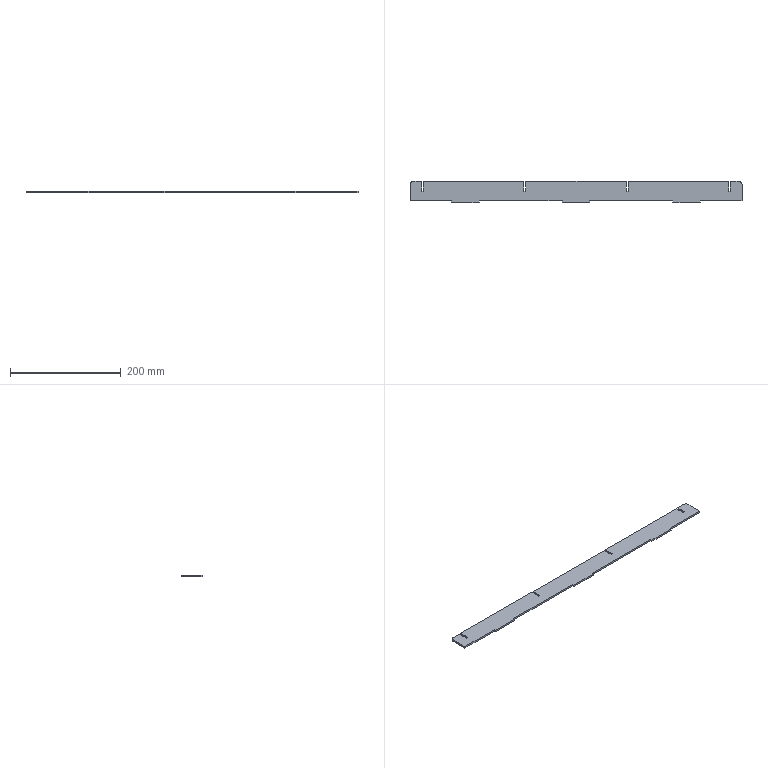Part | SolidWorks | features FlatPattern 1, SMBaseFlange 1, SheetMetal 1 | 1 solid | 36 faces | box 600 x 38 x 3.2 mm | volume 67879 mm3 | plane 34 | cylinder 2 | commonest cylinder face diameters 10 x2
STEP:
#1=CARTESIAN_POINT('',(254.609,-214.8,0.));
#2=VERTEX_POINT('',#1);
#3=CARTESIAN_POINT('',(254.609,-184.8,0.));
#4=VERTEX_POINT('',#3);
#5=CARTESIAN_POINT('',(254.609,-214.8,0.));
#6=DIRECTION('',(0.,1.,0.));
#7=VECTOR('',#6,1000.);
#8=LINE('',#5,#7);
#9=EDGE_CURVE('',#2,#4,#8,.T.);
#10=ORIENTED_EDGE('',*,*,#9,.F.);
#11=CARTESIAN_POINT('',(254.609,-214.8,-3.2));
#12=VERTEX_POINT('',#11);
#13=CARTESIAN_POINT('',(254.609,-214.8,-3.2));
#14=DIRECTION('',(0.,0.,1.));
#15=VECTOR('',#14,1000.);
#16=LINE('',#13,#15);
#17=EDGE_CURVE('',#12,#2,#16,.T.);
#18=ORIENTED_EDGE('',*,*,#17,.F.);
#19=CARTESIAN_POINT('',(254.609,-184.8,-3.2));
#20=VERTEX_POINT('',#19);
#21=CARTESIAN_POINT('',(254.609,-214.8,-3.2));
#22=DIRECTION('',(0.,1.,0.));
#23=VECTOR('',#22,1000.);
#24=LINE('',#21,#23);
#25=EDGE_CURVE('',#12,#20,#24,.T.);
#26=ORIENTED_EDGE('',*,*,#25,.T.);
#27=CARTESIAN_POINT('',(254.609,-184.8,-3.2));
#28=DIRECTION('',(0.,0.,1.));
#29=VECTOR('',#28,1000.);
#30=LINE('',#27,#29);
#31=EDGE_CURVE('',#20,#4,#30,.T.);
#32=ORIENTED_EDGE('',*,*,#31,.T.);
#33=EDGE_LOOP('',(#10,#18,#26,#32));
#34=FACE_OUTER_BOUND('',#33,.T.);
#35=CARTESIAN_POINT('',(254.609,-214.8,-3.2));
#36=DIRECTION('',(1.,0.,0.));
#37=DIRECTION('',(0.,0.,-1.));
#38=AXIS2_PLACEMENT_3D('',#35,#36,#37);
#39=PLANE('',#38);
#40=ADVANCED_FACE('',(#34),#39,.T.);
#41=CARTESIAN_POINT('',(179.609,-214.8,0.));
#42=VERTEX_POINT('',#41);
#43=CARTESIAN_POINT('',(254.609,-214.8,0.));
#44=DIRECTION('',(1.,0.,0.));
#45=VECTOR('',#44,1000.);
#46=LINE('',#43,#45);
#47=EDGE_CURVE('',#42,#2,#46,.T.);
#48=ORIENTED_EDGE('',*,*,#47,.F.);
#49=CARTESIAN_POINT('',(179.609,-214.8,-3.2));
#50=VERTEX_POINT('',#49);
#51=CARTESIAN_POINT('',(179.609,-214.8,-3.2));
#52=DIRECTION('',(0.,0.,1.));
#53=VECTOR('',#52,1000.);
#54=LINE('',#51,#53);
#55=EDGE_CURVE('',#50,#42,#54,.T.);
#56=ORIENTED_EDGE('',*,*,#55,.F.);
#57=CARTESIAN_POINT('',(254.609,-214.8,-3.2));
#58=DIRECTION('',(1.,0.,0.));
#59=VECTOR('',#58,1000.);
#60=LINE('',#57,#59);
#61=EDGE_CURVE('',#50,#12,#60,.T.);
#62=ORIENTED_EDGE('',*,*,#61,.T.);
#63=ORIENTED_EDGE('',*,*,#17,.T.);
#64=EDGE_LOOP('',(#48,#56,#62,#63));
#65=FACE_OUTER_BOUND('',#64,.T.);
#66=CARTESIAN_POINT('',(254.609,-214.8,-3.2));
#67=DIRECTION('',(0.,-1.,0.));
#68=DIRECTION('',(1.,0.,0.));
#69=AXIS2_PLACEMENT_3D('',#66,#67,#68);
#70=PLANE('',#69);
#71=ADVANCED_FACE('',(#65),#70,.T.);
#72=CARTESIAN_POINT('',(179.609,-217.8,0.));
#73=VERTEX_POINT('',#72);
#74=CARTESIAN_POINT('',(179.609,-214.8,0.));
#75=DIRECTION('',(0.,1.,0.));
#76=VECTOR('',#75,1000.);
#77=LINE('',#74,#76);
#78=EDGE_CURVE('',#73,#42,#77,.T.);
#79=ORIENTED_EDGE('',*,*,#78,.F.);
#80=CARTESIAN_POINT('',(179.609,-217.8,-3.2));
#81=VERTEX_POINT('',#80);
#82=CARTESIAN_POINT('',(179.609,-217.8,-3.2));
#83=DIRECTION('',(0.,0.,1.));
#84=VECTOR('',#83,1000.);
#85=LINE('',#82,#84);
#86=EDGE_CURVE('',#81,#73,#85,.T.);
#87=ORIENTED_EDGE('',*,*,#86,.F.);
#88=CARTESIAN_POINT('',(179.609,-214.8,-3.2));
#89=DIRECTION('',(0.,1.,0.));
#90=VECTOR('',#89,1000.);
#91=LINE('',#88,#90);
#92=EDGE_CURVE('',#81,#50,#91,.T.);
#93=ORIENTED_EDGE('',*,*,#92,.T.);
#94=ORIENTED_EDGE('',*,*,#55,.T.);
#95=EDGE_LOOP('',(#79,#87,#93,#94));
#96=FACE_OUTER_BOUND('',#95,.T.);
#97=CARTESIAN_POINT('',(179.609,-214.8,-3.2));
#98=DIRECTION('',(1.,0.,0.));
#99=DIRECTION('',(0.,0.,-1.));
#100=AXIS2_PLACEMENT_3D('',#97,#98,#99);
#101=PLANE('',#100);
#102=ADVANCED_FACE('',(#96),#101,.T.);
#103=CARTESIAN_POINT('',(129.609,-217.8,0.));
#104=VERTEX_POINT('',#103);
#105=CARTESIAN_POINT('',(179.609,-217.8,0.));
#106=DIRECTION('',(1.,0.,0.));
#107=VECTOR('',#106,1000.);
#108=LINE('',#105,#107);
#109=EDGE_CURVE('',#104,#73,#108,.T.);
#110=ORIENTED_EDGE('',*,*,#109,.F.);
#111=CARTESIAN_POINT('',(129.609,-217.8,-3.2));
#112=VERTEX_POINT('',#111);
#113=CARTESIAN_POINT('',(129.609,-217.8,-3.2));
#114=DIRECTION('',(0.,0.,1.));
#115=VECTOR('',#114,1000.);
#116=LINE('',#113,#115);
#117=EDGE_CURVE('',#112,#104,#116,.T.);
#118=ORIENTED_EDGE('',*,*,#117,.F.);
#119=CARTESIAN_POINT('',(179.609,-217.8,-3.2));
#120=DIRECTION('',(1.,0.,0.));
#121=VECTOR('',#120,1000.);
#122=LINE('',#119,#121);
#123=EDGE_CURVE('',#112,#81,#122,.T.);
#124=ORIENTED_EDGE('',*,*,#123,.T.);
#125=ORIENTED_EDGE('',*,*,#86,.T.);
#126=EDGE_LOOP('',(#110,#118,#124,#125));
#127=FACE_OUTER_BOUND('',#126,.T.);
#128=CARTESIAN_POINT('',(179.609,-217.8,-3.2));
#129=DIRECTION('',(0.,-1.,0.));
#130=DIRECTION('',(1.,0.,0.));
#131=AXIS2_PLACEMENT_3D('',#128,#129,#130);
#132=PLANE('',#131);
#133=ADVANCED_FACE('',(#127),#132,.T.);
#134=CARTESIAN_POINT('',(129.609,-214.8,0.));
#135=VERTEX_POINT('',#134);
#136=CARTESIAN_POINT('',(129.609,-217.8,0.));
#137=DIRECTION('',(0.,-1.,0.));
#138=VECTOR('',#137,1000.);
#139=LINE('',#136,#138);
#140=EDGE_CURVE('',#135,#104,#139,.T.);
#141=ORIENTED_EDGE('',*,*,#140,.F.);
#142=CARTESIAN_POINT('',(129.609,-214.8,-3.2));
#143=VERTEX_POINT('',#142);
#144=CARTESIAN_POINT('',(129.609,-214.8,-3.2));
#145=DIRECTION('',(0.,0.,1.));
#146=VECTOR('',#145,1000.);
#147=LINE('',#144,#146);
#148=EDGE_CURVE('',#143,#135,#147,.T.);
#149=ORIENTED_EDGE('',*,*,#148,.F.);
#150=CARTESIAN_POINT('',(129.609,-217.8,-3.2));
#151=DIRECTION('',(0.,-1.,0.));
#152=VECTOR('',#151,1000.);
#153=LINE('',#150,#152);
#154=EDGE_CURVE('',#143,#112,#153,.T.);
#155=ORIENTED_EDGE('',*,*,#154,.T.);
#156=ORIENTED_EDGE('',*,*,#117,.T.);
#157=EDGE_LOOP('',(#141,#149,#155,#156));
#158=FACE_OUTER_BOUND('',#157,.T.);
#159=CARTESIAN_POINT('',(129.609,-217.8,-3.2));
#160=DIRECTION('',(-1.,0.,0.));
#161=DIRECTION('',(0.,0.,1.));
#162=AXIS2_PLACEMENT_3D('',#159,#160,#161);
#163=PLANE('',#162);
#164=ADVANCED_FACE('',(#158),#163,.T.);
#165=CARTESIAN_POINT('',(-20.391,-214.8,0.));
#166=VERTEX_POINT('',#165);
#167=CARTESIAN_POINT('',(129.609,-214.8,0.));
#168=DIRECTION('',(1.,0.,0.));
#169=VECTOR('',#168,1000.);
#170=LINE('',#167,#169);
#171=EDGE_CURVE('',#166,#135,#170,.T.);
#172=ORIENTED_EDGE('',*,*,#171,.F.);
#173=CARTESIAN_POINT('',(-20.391,-214.8,-3.2));
#174=VERTEX_POINT('',#173);
#175=CARTESIAN_POINT('',(-20.391,-214.8,-3.2));
#176=DIRECTION('',(0.,0.,1.));
#177=VECTOR('',#176,1000.);
#178=LINE('',#175,#177);
#179=EDGE_CURVE('',#174,#166,#178,.T.);
#180=ORIENTED_EDGE('',*,*,#179,.F.);
#181=CARTESIAN_POINT('',(129.609,-214.8,-3.2));
#182=DIRECTION('',(1.,0.,0.));
#183=VECTOR('',#182,1000.);
#184=LINE('',#181,#183);
#185=EDGE_CURVE('',#174,#143,#184,.T.);
#186=ORIENTED_EDGE('',*,*,#185,.T.);
#187=ORIENTED_EDGE('',*,*,#148,.T.);
#188=EDGE_LOOP('',(#172,#180,#186,#187));
#189=FACE_OUTER_BOUND('',#188,.T.);
#190=CARTESIAN_POINT('',(129.609,-214.8,-3.2));
#191=DIRECTION('',(0.,-1.,0.));
#192=DIRECTION('',(0.,0.,-1.));
#193=AXIS2_PLACEMENT_3D('',#190,#191,#192);
#194=PLANE('',#193);
#195=ADVANCED_FACE('',(#189),#194,.T.);
#196=CARTESIAN_POINT('',(-20.391,-217.8,0.));
#197=VERTEX_POINT('',#196);
#198=CARTESIAN_POINT('',(-20.391,-214.8,0.));
#199=DIRECTION('',(0.,1.,0.));
#200=VECTOR('',#199,1000.);
#201=LINE('',#198,#200);
#202=EDGE_CURVE('',#197,#166,#201,.T.);
#203=ORIENTED_EDGE('',*,*,#202,.F.);
#204=CARTESIAN_POINT('',(-20.391,-217.8,-3.2));
#205=VERTEX_POINT('',#204);
#206=CARTESIAN_POINT('',(-20.391,-217.8,-3.2));
#207=DIRECTION('',(0.,0.,1.));
#208=VECTOR('',#207,1000.);
#209=LINE('',#206,#208);
#210=EDGE_CURVE('',#205,#197,#209,.T.);
#211=ORIENTED_EDGE('',*,*,#210,.F.);
#212=CARTESIAN_POINT('',(-20.391,-214.8,-3.2));
#213=DIRECTION('',(0.,1.,0.));
#214=VECTOR('',#213,1000.);
#215=LINE('',#212,#214);
#216=EDGE_CURVE('',#205,#174,#215,.T.);
#217=ORIENTED_EDGE('',*,*,#216,.T.);
#218=ORIENTED_EDGE('',*,*,#179,.T.);
#219=EDGE_LOOP('',(#203,#211,#217,#218));
#220=FACE_OUTER_BOUND('',#219,.T.);
#221=CARTESIAN_POINT('',(-20.391,-214.8,-3.2));
#222=DIRECTION('',(1.,0.,0.));
#223=DIRECTION('',(0.,1.,0.));
#224=AXIS2_PLACEMENT_3D('',#221,#222,#223);
#225=PLANE('',#224);
#226=ADVANCED_FACE('',(#220),#225,.T.);
#227=CARTESIAN_POINT('',(-70.391,-217.8,0.));
#228=VERTEX_POINT('',#227);
#229=CARTESIAN_POINT('',(-20.391,-217.8,0.));
#230=DIRECTION('',(1.,0.,0.));
#231=VECTOR('',#230,1000.);
#232=LINE('',#229,#231);
#233=EDGE_CURVE('',#228,#197,#232,.T.);
#234=ORIENTED_EDGE('',*,*,#233,.F.);
#235=CARTESIAN_POINT('',(-70.391,-217.8,-3.2));
#236=VERTEX_POINT('',#235);
#237=CARTESIAN_POINT('',(-70.391,-217.8,-3.2));
#238=DIRECTION('',(0.,0.,1.));
#239=VECTOR('',#238,1000.);
#240=LINE('',#237,#239);
#241=EDGE_CURVE('',#236,#228,#240,.T.);
#242=ORIENTED_EDGE('',*,*,#241,.F.);
#243=CARTESIAN_POINT('',(-20.391,-217.8,-3.2));
#244=DIRECTION('',(1.,0.,0.));
#245=VECTOR('',#244,1000.);
#246=LINE('',#243,#245);
#247=EDGE_CURVE('',#236,#205,#246,.T.);
#248=ORIENTED_EDGE('',*,*,#247,.T.);
#249=ORIENTED_EDGE('',*,*,#210,.T.);
#250=EDGE_LOOP('',(#234,#242,#248,#249));
#251=FACE_OUTER_BOUND('',#250,.T.);
#252=CARTESIAN_POINT('',(-20.391,-217.8,-3.2));
#253=DIRECTION('',(0.,-1.,0.));
#254=DIRECTION('',(0.,0.,-1.));
#255=AXIS2_PLACEMENT_3D('',#252,#253,#254);
#256=PLANE('',#255);
#257=ADVANCED_FACE('',(#251),#256,.T.);
#258=CARTESIAN_POINT('',(-70.391,-214.8,0.));
#259=VERTEX_POINT('',#258);
#260=CARTESIAN_POINT('',(-70.391,-217.8,0.));
#261=DIRECTION('',(0.,-1.,0.));
#262=VECTOR('',#261,1000.);
#263=LINE('',#260,#262);
#264=EDGE_CURVE('',#259,#228,#263,.T.);
#265=ORIENTED_EDGE('',*,*,#264,.F.);
#266=CARTESIAN_POINT('',(-70.391,-214.8,-3.2));
#267=VERTEX_POINT('',#266);
#268=CARTESIAN_POINT('',(-70.391,-214.8,-3.2));
#269=DIRECTION('',(0.,0.,1.));
#270=VECTOR('',#269,1000.);
#271=LINE('',#268,#270);
#272=EDGE_CURVE('',#267,#259,#271,.T.);
#273=ORIENTED_EDGE('',*,*,#272,.F.);
#274=CARTESIAN_POINT('',(-70.391,-217.8,-3.2));
#275=DIRECTION('',(0.,-1.,0.));
#276=VECTOR('',#275,1000.);
#277=LINE('',#274,#276);
#278=EDGE_CURVE('',#267,#236,#277,.T.);
#279=ORIENTED_EDGE('',*,*,#278,.T.);
#280=ORIENTED_EDGE('',*,*,#241,.T.);
#281=EDGE_LOOP('',(#265,#273,#279,#280));
#282=FACE_OUTER_BOUND('',#281,.T.);
#283=CARTESIAN_POINT('',(-70.391,-217.8,-3.2));
#284=DIRECTION('',(-1.,0.,0.));
#285=DIRECTION('',(0.,0.,1.));
#286=AXIS2_PLACEMENT_3D('',#283,#284,#285);
#287=PLANE('',#286);
#288=ADVANCED_FACE('',(#282),#287,.T.);
#289=CARTESIAN_POINT('',(-220.391,-214.8,0.));
#290=VERTEX_POINT('',#289);
#291=CARTESIAN_POINT('',(-70.391,-214.8,0.));
#292=DIRECTION('',(1.,0.,0.));
#293=VECTOR('',#292,1000.);
#294=LINE('',#291,#293);
#295=EDGE_CURVE('',#290,#259,#294,.T.);
#296=ORIENTED_EDGE('',*,*,#295,.F.);
#297=CARTESIAN_POINT('',(-220.391,-214.8,-3.2));
#298=VERTEX_POINT('',#297);
#299=CARTESIAN_POINT('',(-220.391,-214.8,-3.2));
#300=DIRECTION('',(0.,0.,1.));
#301=VECTOR('',#300,1000.);
#302=LINE('',#299,#301);
#303=EDGE_CURVE('',#298,#290,#302,.T.);
#304=ORIENTED_EDGE('',*,*,#303,.F.);
#305=CARTESIAN_POINT('',(-70.391,-214.8,-3.2));
#306=DIRECTION('',(1.,0.,0.));
#307=VECTOR('',#306,1000.);
#308=LINE('',#305,#307);
#309=EDGE_CURVE('',#298,#267,#308,.T.);
#310=ORIENTED_EDGE('',*,*,#309,.T.);
#311=ORIENTED_EDGE('',*,*,#272,.T.);
#312=EDGE_LOOP('',(#296,#304,#310,#311));
#313=FACE_OUTER_BOUND('',#312,.T.);
#314=CARTESIAN_POINT('',(-70.391,-214.8,-3.2));
#315=DIRECTION('',(0.,-1.,0.));
#316=DIRECTION('',(0.,0.,-1.));
#317=AXIS2_PLACEMENT_3D('',#314,#315,#316);
#318=PLANE('',#317);
#319=ADVANCED_FACE('',(#313),#318,.T.);
#320=CARTESIAN_POINT('',(-220.391,-217.8,0.));
#321=VERTEX_POINT('',#320);
#322=CARTESIAN_POINT('',(-220.391,-217.8,0.));
#323=DIRECTION('',(0.,1.,0.));
#324=VECTOR('',#323,1000.);
#325=LINE('',#322,#324);
#326=EDGE_CURVE('',#321,#290,#325,.T.);
#327=ORIENTED_EDGE('',*,*,#326,.F.);
#328=CARTESIAN_POINT('',(-220.391,-217.8,-3.2));
#329=VERTEX_POINT('',#328);
#330=CARTESIAN_POINT('',(-220.391,-217.8,-3.2));
#331=DIRECTION('',(0.,0.,1.));
#332=VECTOR('',#331,1000.);
#333=LINE('',#330,#332);
#334=EDGE_CURVE('',#329,#321,#333,.T.);
#335=ORIENTED_EDGE('',*,*,#334,.F.);
#336=CARTESIAN_POINT('',(-220.391,-217.8,-3.2));
#337=DIRECTION('',(0.,1.,0.));
#338=VECTOR('',#337,1000.);
#339=LINE('',#336,#338);
#340=EDGE_CURVE('',#329,#298,#339,.T.);
#341=ORIENTED_EDGE('',*,*,#340,.T.);
#342=ORIENTED_EDGE('',*,*,#303,.T.);
#343=EDGE_LOOP('',(#327,#335,#341,#342));
#344=FACE_OUTER_BOUND('',#343,.T.);
#345=CARTESIAN_POINT('',(-220.391,-217.8,-3.2));
#346=DIRECTION('',(1.,0.,0.));
#347=DIRECTION('',(0.,1.,0.));
#348=AXIS2_PLACEMENT_3D('',#345,#346,#347);
#349=PLANE('',#348);
#350=ADVANCED_FACE('',(#344),#349,.T.);
#351=CARTESIAN_POINT('',(-270.391,-217.8,0.));
#352=VERTEX_POINT('',#351);
#353=CARTESIAN_POINT('',(-270.391,-217.8,0.));
#354=DIRECTION('',(1.,0.,0.));
#355=VECTOR('',#354,1000.);
#356=LINE('',#353,#355);
#357=EDGE_CURVE('',#352,#321,#356,.T.);
#358=ORIENTED_EDGE('',*,*,#357,.F.);
#359=CARTESIAN_POINT('',(-270.391,-217.8,-3.2));
#360=VERTEX_POINT('',#359);
#361=CARTESIAN_POINT('',(-270.391,-217.8,-3.2));
#362=DIRECTION('',(0.,0.,1.));
#363=VECTOR('',#362,1000.);
#364=LINE('',#361,#363);
#365=EDGE_CURVE('',#360,#352,#364,.T.);
#366=ORIENTED_EDGE('',*,*,#365,.F.);
#367=CARTESIAN_POINT('',(-270.391,-217.8,-3.2));
#368=DIRECTION('',(1.,0.,0.));
#369=VECTOR('',#368,1000.);
#370=LINE('',#367,#369);
#371=EDGE_CURVE('',#360,#329,#370,.T.);
#372=ORIENTED_EDGE('',*,*,#371,.T.);
#373=ORIENTED_EDGE('',*,*,#334,.T.);
#374=EDGE_LOOP('',(#358,#366,#372,#373));
#375=FACE_OUTER_BOUND('',#374,.T.);
#376=CARTESIAN_POINT('',(-270.391,-217.8,-3.2));
#377=DIRECTION('',(0.,-1.,0.));
#378=DIRECTION('',(0.,0.,-1.));
#379=AXIS2_PLACEMENT_3D('',#376,#377,#378);
#380=PLANE('',#379);
#381=ADVANCED_FACE('',(#375),#380,.T.);
#382=CARTESIAN_POINT('',(-270.391,-214.8,0.));
#383=VERTEX_POINT('',#382);
#384=CARTESIAN_POINT('',(-270.391,-214.8,0.));
#385=DIRECTION('',(0.,-1.,0.));
#386=VECTOR('',#385,1000.);
#387=LINE('',#384,#386);
#388=EDGE_CURVE('',#383,#352,#387,.T.);
#389=ORIENTED_EDGE('',*,*,#388,.F.);
#390=CARTESIAN_POINT('',(-270.391,-214.8,-3.2));
#391=VERTEX_POINT('',#390);
#392=CARTESIAN_POINT('',(-270.391,-214.8,-3.2));
#393=DIRECTION('',(0.,0.,1.));
#394=VECTOR('',#393,1000.);
#395=LINE('',#392,#394);
#396=EDGE_CURVE('',#391,#383,#395,.T.);
#397=ORIENTED_EDGE('',*,*,#396,.F.);
#398=CARTESIAN_POINT('',(-270.391,-214.8,-3.2));
#399=DIRECTION('',(0.,-1.,0.));
#400=VECTOR('',#399,1000.);
#401=LINE('',#398,#400);
#402=EDGE_CURVE('',#391,#360,#401,.T.);
#403=ORIENTED_EDGE('',*,*,#402,.T.);
#404=ORIENTED_EDGE('',*,*,#365,.T.);
#405=EDGE_LOOP('',(#389,#397,#403,#404));
#406=FACE_OUTER_BOUND('',#405,.T.);
#407=CARTESIAN_POINT('',(-270.391,-214.8,-3.2));
#408=DIRECTION('',(-1.,0.,0.));
#409=DIRECTION('',(0.,0.,1.));
#410=AXIS2_PLACEMENT_3D('',#407,#408,#409);
#411=PLANE('',#410);
#412=ADVANCED_FACE('',(#406),#411,.T.);
#413=CARTESIAN_POINT('',(-345.391,-214.8,0.));
#414=VERTEX_POINT('',#413);
#415=CARTESIAN_POINT('',(-270.391,-214.8,0.));
#416=DIRECTION('',(1.,0.,0.));
#417=VECTOR('',#416,1000.);
#418=LINE('',#415,#417);
#419=EDGE_CURVE('',#414,#383,#418,.T.);
#420=ORIENTED_EDGE('',*,*,#419,.F.);
#421=CARTESIAN_POINT('',(-345.391,-214.8,-3.2));
#422=VERTEX_POINT('',#421);
#423=CARTESIAN_POINT('',(-345.391,-214.8,-3.2));
#424=DIRECTION('',(0.,0.,1.));
#425=VECTOR('',#424,1000.);
#426=LINE('',#423,#425);
#427=EDGE_CURVE('',#422,#414,#426,.T.);
#428=ORIENTED_EDGE('',*,*,#427,.F.);
#429=CARTESIAN_POINT('',(-270.391,-214.8,-3.2));
#430=DIRECTION('',(1.,0.,0.));
#431=VECTOR('',#430,1000.);
#432=LINE('',#429,#431);
#433=EDGE_CURVE('',#422,#391,#432,.T.);
#434=ORIENTED_EDGE('',*,*,#433,.T.);
#435=ORIENTED_EDGE('',*,*,#396,.T.);
#436=EDGE_LOOP('',(#420,#428,#434,#435));
#437=FACE_OUTER_BOUND('',#436,.T.);
#438=CARTESIAN_POINT('',(-270.391,-214.8,-3.2));
#439=DIRECTION('',(0.,-1.,0.));
#440=DIRECTION('',(1.,0.,0.));
#441=AXIS2_PLACEMENT_3D('',#438,#439,#440);
#442=PLANE('',#441);
#443=ADVANCED_FACE('',(#437),#442,.T.);
#444=CARTESIAN_POINT('',(-345.391,-184.8,0.));
#445=VERTEX_POINT('',#444);
#446=CARTESIAN_POINT('',(-345.391,-214.8,0.));
#447=DIRECTION('',(0.,-1.,0.));
#448=VECTOR('',#447,1000.);
#449=LINE('',#446,#448);
#450=EDGE_CURVE('',#445,#414,#449,.T.);
#451=ORIENTED_EDGE('',*,*,#450,.F.);
#452=CARTESIAN_POINT('',(-345.391,-184.8,-3.2));
#453=VERTEX_POINT('',#452);
#454=CARTESIAN_POINT('',(-345.391,-184.8,-3.2));
#455=DIRECTION('',(0.,0.,1.));
#456=VECTOR('',#455,1000.);
#457=LINE('',#454,#456);
#458=EDGE_CURVE('',#453,#445,#457,.T.);
#459=ORIENTED_EDGE('',*,*,#458,.F.);
#460=CARTESIAN_POINT('',(-345.391,-214.8,-3.2));
#461=DIRECTION('',(0.,-1.,0.));
#462=VECTOR('',#461,1000.);
#463=LINE('',#460,#462);
#464=EDGE_CURVE('',#453,#422,#463,.T.);
#465=ORIENTED_EDGE('',*,*,#464,.T.);
#466=ORIENTED_EDGE('',*,*,#427,.T.);
#467=EDGE_LOOP('',(#451,#459,#465,#466));
#468=FACE_OUTER_BOUND('',#467,.T.);
#469=CARTESIAN_POINT('',(-345.391,-214.8,-3.2));
#470=DIRECTION('',(-1.,0.,0.));
#471=DIRECTION('',(0.,0.,1.));
#472=AXIS2_PLACEMENT_3D('',#469,#470,#471);
#473=PLANE('',#472);
#474=ADVANCED_FACE('',(#468),#473,.T.);
#475=CARTESIAN_POINT('',(-340.391,-179.8,0.));
#476=VERTEX_POINT('',#475);
#477=CARTESIAN_POINT('',(-340.391,-184.8,0.));
#478=DIRECTION('',(0.,0.,1.));
#479=DIRECTION('',(1.,0.,0.));
#480=AXIS2_PLACEMENT_3D('',#477,#478,#479);
#481=CIRCLE('',#480,5.);
#482=EDGE_CURVE('',#476,#445,#481,.T.);
#483=ORIENTED_EDGE('',*,*,#482,.F.);
#484=CARTESIAN_POINT('',(-340.391,-179.8,-3.2));
#485=VERTEX_POINT('',#484);
#486=CARTESIAN_POINT('',(-340.391,-179.8,-3.2));
#487=DIRECTION('',(0.,0.,1.));
#488=VECTOR('',#487,1000.);
#489=LINE('',#486,#488);
#490=EDGE_CURVE('',#485,#476,#489,.T.);
#491=ORIENTED_EDGE('',*,*,#490,.F.);
#492=CARTESIAN_POINT('',(-340.391,-184.8,-3.2));
#493=DIRECTION('',(0.,0.,1.));
#494=DIRECTION('',(1.,0.,0.));
#495=AXIS2_PLACEMENT_3D('',#492,#493,#494);
#496=CIRCLE('',#495,5.);
#497=EDGE_CURVE('',#485,#453,#496,.T.);
#498=ORIENTED_EDGE('',*,*,#497,.T.);
#499=ORIENTED_EDGE('',*,*,#458,.T.);
#500=EDGE_LOOP('',(#483,#491,#498,#499));
#501=FACE_OUTER_BOUND('',#500,.T.);
#502=CARTESIAN_POINT('',(-340.391,-184.8,-3.2));
#503=DIRECTION('',(0.,0.,1.));
#504=DIRECTION('',(1.,0.,0.));
#505=AXIS2_PLACEMENT_3D('',#502,#503,#504);
#506=CYLINDRICAL_SURFACE('',#505,5.);
#507=ADVANCED_FACE('',(#501),#506,.T.);
#508=CARTESIAN_POINT('',(-324.491,-179.8,0.));
#509=VERTEX_POINT('',#508);
#510=CARTESIAN_POINT('',(-324.491,-179.8,0.));
#511=DIRECTION('',(-1.,0.,0.));
#512=VECTOR('',#511,1000.);
#513=LINE('',#510,#512);
#514=EDGE_CURVE('',#509,#476,#513,.T.);
#515=ORIENTED_EDGE('',*,*,#514,.F.);
#516=CARTESIAN_POINT('',(-324.491,-179.8,-3.2));
#517=VERTEX_POINT('',#516);
#518=CARTESIAN_POINT('',(-324.491,-179.8,-3.2));
#519=DIRECTION('',(0.,0.,1.));
#520=VECTOR('',#519,1000.);
#521=LINE('',#518,#520);
#522=EDGE_CURVE('',#517,#509,#521,.T.);
#523=ORIENTED_EDGE('',*,*,#522,.F.);
#524=CARTESIAN_POINT('',(-324.491,-179.8,-3.2));
#525=DIRECTION('',(-1.,0.,0.));
#526=VECTOR('',#525,1000.);
#527=LINE('',#524,#526);
#528=EDGE_CURVE('',#517,#485,#527,.T.);
#529=ORIENTED_EDGE('',*,*,#528,.T.);
#530=ORIENTED_EDGE('',*,*,#490,.T.);
#531=EDGE_LOOP('',(#515,#523,#529,#530));
#532=FACE_OUTER_BOUND('',#531,.T.);
#533=CARTESIAN_POINT('',(-324.491,-179.8,-3.2));
#534=DIRECTION('',(0.,1.,0.));
#535=DIRECTION('',(-1.,0.,0.));
#536=AXIS2_PLACEMENT_3D('',#533,#534,#535);
#537=PLANE('',#536);
#538=ADVANCED_FACE('',(#532),#537,.T.);
#539=CARTESIAN_POINT('',(-324.491,-197.55,0.));
#540=VERTEX_POINT('',#539);
#541=CARTESIAN_POINT('',(-324.491,-197.55,0.));
#542=DIRECTION('',(0.,1.,0.));
#543=VECTOR('',#542,1000.);
#544=LINE('',#541,#543);
#545=EDGE_CURVE('',#540,#509,#544,.T.);
#546=ORIENTED_EDGE('',*,*,#545,.F.);
#547=CARTESIAN_POINT('',(-324.491,-197.55,-3.2));
#548=VERTEX_POINT('',#547);
#549=CARTESIAN_POINT('',(-324.491,-197.55,-3.2));
#550=DIRECTION('',(0.,0.,1.));
#551=VECTOR('',#550,1000.);
#552=LINE('',#549,#551);
#553=EDGE_CURVE('',#548,#540,#552,.T.);
#554=ORIENTED_EDGE('',*,*,#553,.F.);
#555=CARTESIAN_POINT('',(-324.491,-197.55,-3.2));
#556=DIRECTION('',(0.,1.,0.));
#557=VECTOR('',#556,1000.);
#558=LINE('',#555,#557);
#559=EDGE_CURVE('',#548,#517,#558,.T.);
#560=ORIENTED_EDGE('',*,*,#559,.T.);
#561=ORIENTED_EDGE('',*,*,#522,.T.);
#562=EDGE_LOOP('',(#546,#554,#560,#561));
#563=FACE_OUTER_BOUND('',#562,.T.);
#564=CARTESIAN_POINT('',(-324.491,-197.55,-3.2));
#565=DIRECTION('',(1.,0.,0.));
#566=DIRECTION('',(0.,1.,0.));
#567=AXIS2_PLACEMENT_3D('',#564,#565,#566);
#568=PLANE('',#567);
#569=ADVANCED_FACE('',(#563),#568,.T.);
#570=CARTESIAN_POINT('',(-321.291,-197.55,0.));
#571=VERTEX_POINT('',#570);
#572=CARTESIAN_POINT('',(-321.291,-197.55,0.));
#573=DIRECTION('',(-1.,0.,0.));
#574=VECTOR('',#573,1000.);
#575=LINE('',#572,#574);
#576=EDGE_CURVE('',#571,#540,#575,.T.);
#577=ORIENTED_EDGE('',*,*,#576,.F.);
#578=CARTESIAN_POINT('',(-321.291,-197.55,-3.2));
#579=VERTEX_POINT('',#578);
#580=CARTESIAN_POINT('',(-321.291,-197.55,-3.2));
#581=DIRECTION('',(0.,0.,1.));
#582=VECTOR('',#581,1000.);
#583=LINE('',#580,#582);
#584=EDGE_CURVE('',#579,#571,#583,.T.);
#585=ORIENTED_EDGE('',*,*,#584,.F.);
#586=CARTESIAN_POINT('',(-321.291,-197.55,-3.2));
#587=DIRECTION('',(-1.,0.,0.));
#588=VECTOR('',#587,1000.);
#589=LINE('',#586,#588);
#590=EDGE_CURVE('',#579,#548,#589,.T.);
#591=ORIENTED_EDGE('',*,*,#590,.T.);
#592=ORIENTED_EDGE('',*,*,#553,.T.);
#593=EDGE_LOOP('',(#577,#585,#591,#592));
#594=FACE_OUTER_BOUND('',#593,.T.);
#595=CARTESIAN_POINT('',(-321.291,-197.55,-3.2));
#596=DIRECTION('',(0.,1.,0.));
#597=DIRECTION('',(0.,0.,1.));
#598=AXIS2_PLACEMENT_3D('',#595,#596,#597);
#599=PLANE('',#598);
#600=ADVANCED_FACE('',(#594),#599,.T.);
#601=CARTESIAN_POINT('',(-321.291,-179.8,0.));
#602=VERTEX_POINT('',#601);
#603=CARTESIAN_POINT('',(-321.291,-179.8,0.));
#604=DIRECTION('',(0.,-1.,0.));
#605=VECTOR('',#604,1000.);
#606=LINE('',#603,#605);
#607=EDGE_CURVE('',#602,#571,#606,.T.);
#608=ORIENTED_EDGE('',*,*,#607,.F.);
#609=CARTESIAN_POINT('',(-321.291,-179.8,-3.2));
#610=VERTEX_POINT('',#609);
#611=CARTESIAN_POINT('',(-321.291,-179.8,-3.2));
#612=DIRECTION('',(0.,0.,1.));
#613=VECTOR('',#612,1000.);
#614=LINE('',#611,#613);
#615=EDGE_CURVE('',#610,#602,#614,.T.);
#616=ORIENTED_EDGE('',*,*,#615,.F.);
#617=CARTESIAN_POINT('',(-321.291,-179.8,-3.2));
#618=DIRECTION('',(0.,-1.,0.));
#619=VECTOR('',#618,1000.);
#620=LINE('',#617,#619);
#621=EDGE_CURVE('',#610,#579,#620,.T.);
#622=ORIENTED_EDGE('',*,*,#621,.T.);
#623=ORIENTED_EDGE('',*,*,#584,.T.);
#624=EDGE_LOOP('',(#608,#616,#622,#623));
#625=FACE_OUTER_BOUND('',#624,.T.);
#626=CARTESIAN_POINT('',(-321.291,-179.8,-3.2));
#627=DIRECTION('',(-1.,0.,0.));
#628=DIRECTION('',(0.,-1.,0.));
#629=AXIS2_PLACEMENT_3D('',#626,#627,#628);
#630=PLANE('',#629);
#631=ADVANCED_FACE('',(#625),#630,.T.);
#632=CARTESIAN_POINT('',(-139.491,-179.8,0.));
#633=VERTEX_POINT('',#632);
#634=CARTESIAN_POINT('',(-139.491,-179.8,0.));
#635=DIRECTION('',(-1.,0.,0.));
#636=VECTOR('',#635,1000.);
#637=LINE('',#634,#636);
#638=EDGE_CURVE('',#633,#602,#637,.T.);
#639=ORIENTED_EDGE('',*,*,#638,.F.);
#640=CARTESIAN_POINT('',(-139.491,-179.8,-3.2));
#641=VERTEX_POINT('',#640);
#642=CARTESIAN_POINT('',(-139.491,-179.8,-3.2));
#643=DIRECTION('',(0.,0.,1.));
#644=VECTOR('',#643,1000.);
#645=LINE('',#642,#644);
#646=EDGE_CURVE('',#641,#633,#645,.T.);
#647=ORIENTED_EDGE('',*,*,#646,.F.);
#648=CARTESIAN_POINT('',(-139.491,-179.8,-3.2));
#649=DIRECTION('',(-1.,0.,0.));
#650=VECTOR('',#649,1000.);
#651=LINE('',#648,#650);
#652=EDGE_CURVE('',#641,#610,#651,.T.);
#653=ORIENTED_EDGE('',*,*,#652,.T.);
#654=ORIENTED_EDGE('',*,*,#615,.T.);
#655=EDGE_LOOP('',(#639,#647,#653,#654));
#656=FACE_OUTER_BOUND('',#655,.T.);
#657=CARTESIAN_POINT('',(-139.491,-179.8,-3.2));
#658=DIRECTION('',(0.,1.,0.));
#659=DIRECTION('',(-1.,0.,0.));
#660=AXIS2_PLACEMENT_3D('',#657,#658,#659);
#661=PLANE('',#660);
#662=ADVANCED_FACE('',(#656),#661,.T.);
#663=CARTESIAN_POINT('',(-139.491,-197.55,0.));
#664=VERTEX_POINT('',#663);
#665=CARTESIAN_POINT('',(-139.491,-197.55,0.));
#666=DIRECTION('',(0.,1.,0.));
#667=VECTOR('',#666,1000.);
#668=LINE('',#665,#667);
#669=EDGE_CURVE('',#664,#633,#668,.T.);
#670=ORIENTED_EDGE('',*,*,#669,.F.);
#671=CARTESIAN_POINT('',(-139.491,-197.55,-3.2));
#672=VERTEX_POINT('',#671);
#673=CARTESIAN_POINT('',(-139.491,-197.55,-3.2));
#674=DIRECTION('',(0.,0.,1.));
#675=VECTOR('',#674,1000.);
#676=LINE('',#673,#675);
#677=EDGE_CURVE('',#672,#664,#676,.T.);
#678=ORIENTED_EDGE('',*,*,#677,.F.);
#679=CARTESIAN_POINT('',(-139.491,-197.55,-3.2));
#680=DIRECTION('',(0.,1.,0.));
#681=VECTOR('',#680,1000.);
#682=LINE('',#679,#681);
#683=EDGE_CURVE('',#672,#641,#682,.T.);
#684=ORIENTED_EDGE('',*,*,#683,.T.);
#685=ORIENTED_EDGE('',*,*,#646,.T.);
#686=EDGE_LOOP('',(#670,#678,#684,#685));
#687=FACE_OUTER_BOUND('',#686,.T.);
#688=CARTESIAN_POINT('',(-139.491,-197.55,-3.2));
#689=DIRECTION('',(1.,0.,0.));
#690=DIRECTION('',(0.,1.,0.));
#691=AXIS2_PLACEMENT_3D('',#688,#689,#690);
#692=PLANE('',#691);
#693=ADVANCED_FACE('',(#687),#692,.T.);
#694=CARTESIAN_POINT('',(-136.291,-197.55,0.));
#695=VERTEX_POINT('',#694);
#696=CARTESIAN_POINT('',(-136.291,-197.55,0.));
#697=DIRECTION('',(-1.,0.,0.));
#698=VECTOR('',#697,1000.);
#699=LINE('',#696,#698);
#700=EDGE_CURVE('',#695,#664,#699,.T.);
#701=ORIENTED_EDGE('',*,*,#700,.F.);
#702=CARTESIAN_POINT('',(-136.291,-197.55,-3.2));
#703=VERTEX_POINT('',#702);
#704=CARTESIAN_POINT('',(-136.291,-197.55,-3.2));
#705=DIRECTION('',(0.,0.,1.));
#706=VECTOR('',#705,1000.);
#707=LINE('',#704,#706);
#708=EDGE_CURVE('',#703,#695,#707,.T.);
#709=ORIENTED_EDGE('',*,*,#708,.F.);
#710=CARTESIAN_POINT('',(-136.291,-197.55,-3.2));
#711=DIRECTION('',(-1.,0.,0.));
#712=VECTOR('',#711,1000.);
#713=LINE('',#710,#712);
#714=EDGE_CURVE('',#703,#672,#713,.T.);
#715=ORIENTED_EDGE('',*,*,#714,.T.);
#716=ORIENTED_EDGE('',*,*,#677,.T.);
#717=EDGE_LOOP('',(#701,#709,#715,#716));
#718=FACE_OUTER_BOUND('',#717,.T.);
#719=CARTESIAN_POINT('',(-136.291,-197.55,-3.2));
#720=DIRECTION('',(0.,1.,0.));
#721=DIRECTION('',(0.,0.,1.));
#722=AXIS2_PLACEMENT_3D('',#719,#720,#721);
#723=PLANE('',#722);
#724=ADVANCED_FACE('',(#718),#723,.T.);
#725=CARTESIAN_POINT('',(-136.291,-179.8,0.));
#726=VERTEX_POINT('',#725);
#727=CARTESIAN_POINT('',(-136.291,-179.8,0.));
#728=DIRECTION('',(0.,-1.,0.));
#729=VECTOR('',#728,1000.);
#730=LINE('',#727,#729);
#731=EDGE_CURVE('',#726,#695,#730,.T.);
#732=ORIENTED_EDGE('',*,*,#731,.F.);
#733=CARTESIAN_POINT('',(-136.291,-179.8,-3.2));
#734=VERTEX_POINT('',#733);
#735=CARTESIAN_POINT('',(-136.291,-179.8,-3.2));
#736=DIRECTION('',(0.,0.,1.));
#737=VECTOR('',#736,1000.);
#738=LINE('',#735,#737);
#739=EDGE_CURVE('',#734,#726,#738,.T.);
#740=ORIENTED_EDGE('',*,*,#739,.F.);
#741=CARTESIAN_POINT('',(-136.291,-179.8,-3.2));
#742=DIRECTION('',(0.,-1.,0.));
#743=VECTOR('',#742,1000.);
#744=LINE('',#741,#743);
#745=EDGE_CURVE('',#734,#703,#744,.T.);
#746=ORIENTED_EDGE('',*,*,#745,.T.);
#747=ORIENTED_EDGE('',*,*,#708,.T.);
#748=EDGE_LOOP('',(#732,#740,#746,#747));
#749=FACE_OUTER_BOUND('',#748,.T.);
#750=CARTESIAN_POINT('',(-136.291,-179.8,-3.2));
#751=DIRECTION('',(-1.,0.,0.));
#752=DIRECTION('',(0.,-1.,0.));
#753=AXIS2_PLACEMENT_3D('',#750,#751,#752);
#754=PLANE('',#753);
#755=ADVANCED_FACE('',(#749),#754,.T.);
#756=CARTESIAN_POINT('',(45.509,-179.8,0.));
#757=VERTEX_POINT('',#756);
#758=CARTESIAN_POINT('',(45.509,-179.8,0.));
#759=DIRECTION('',(-1.,0.,0.));
#760=VECTOR('',#759,1000.);
#761=LINE('',#758,#760);
#762=EDGE_CURVE('',#757,#726,#761,.T.);
#763=ORIENTED_EDGE('',*,*,#762,.F.);
#764=CARTESIAN_POINT('',(45.509,-179.8,-3.2));
#765=VERTEX_POINT('',#764);
#766=CARTESIAN_POINT('',(45.509,-179.8,-3.2));
#767=DIRECTION('',(0.,0.,1.));
#768=VECTOR('',#767,1000.);
#769=LINE('',#766,#768);
#770=EDGE_CURVE('',#765,#757,#769,.T.);
#771=ORIENTED_EDGE('',*,*,#770,.F.);
#772=CARTESIAN_POINT('',(45.509,-179.8,-3.2));
#773=DIRECTION('',(-1.,0.,0.));
#774=VECTOR('',#773,1000.);
#775=LINE('',#772,#774);
#776=EDGE_CURVE('',#765,#734,#775,.T.);
#777=ORIENTED_EDGE('',*,*,#776,.T.);
#778=ORIENTED_EDGE('',*,*,#739,.T.);
#779=EDGE_LOOP('',(#763,#771,#777,#778));
#780=FACE_OUTER_BOUND('',#779,.T.);
#781=CARTESIAN_POINT('',(45.509,-179.8,-3.2));
#782=DIRECTION('',(0.,1.,0.));
#783=DIRECTION('',(-1.,0.,0.));
#784=AXIS2_PLACEMENT_3D('',#781,#782,#783);
#785=PLANE('',#784);
#786=ADVANCED_FACE('',(#780),#785,.T.);
#787=CARTESIAN_POINT('',(45.509,-197.55,0.));
#788=VERTEX_POINT('',#787);
#789=CARTESIAN_POINT('',(45.509,-197.55,0.));
#790=DIRECTION('',(0.,1.,0.));
#791=VECTOR('',#790,1000.);
#792=LINE('',#789,#791);
#793=EDGE_CURVE('',#788,#757,#792,.T.);
#794=ORIENTED_EDGE('',*,*,#793,.F.);
#795=CARTESIAN_POINT('',(45.509,-197.55,-3.2));
#796=VERTEX_POINT('',#795);
#797=CARTESIAN_POINT('',(45.509,-197.55,-3.2));
#798=DIRECTION('',(0.,0.,1.));
#799=VECTOR('',#798,1000.);
#800=LINE('',#797,#799);
#801=EDGE_CURVE('',#796,#788,#800,.T.);
#802=ORIENTED_EDGE('',*,*,#801,.F.);
#803=CARTESIAN_POINT('',(45.509,-197.55,-3.2));
#804=DIRECTION('',(0.,1.,0.));
#805=VECTOR('',#804,1000.);
#806=LINE('',#803,#805);
#807=EDGE_CURVE('',#796,#765,#806,.T.);
#808=ORIENTED_EDGE('',*,*,#807,.T.);
#809=ORIENTED_EDGE('',*,*,#770,.T.);
#810=EDGE_LOOP('',(#794,#802,#808,#809));
#811=FACE_OUTER_BOUND('',#810,.T.);
#812=CARTESIAN_POINT('',(45.509,-197.55,-3.2));
#813=DIRECTION('',(1.,0.,0.));
#814=DIRECTION('',(0.,1.,0.));
#815=AXIS2_PLACEMENT_3D('',#812,#813,#814);
#816=PLANE('',#815);
#817=ADVANCED_FACE('',(#811),#816,.T.);
#818=CARTESIAN_POINT('',(48.709,-197.55,0.));
#819=VERTEX_POINT('',#818);
#820=CARTESIAN_POINT('',(48.709,-197.55,0.));
#821=DIRECTION('',(-1.,0.,0.));
#822=VECTOR('',#821,1000.);
#823=LINE('',#820,#822);
#824=EDGE_CURVE('',#819,#788,#823,.T.);
#825=ORIENTED_EDGE('',*,*,#824,.F.);
#826=CARTESIAN_POINT('',(48.709,-197.55,-3.2));
#827=VERTEX_POINT('',#826);
#828=CARTESIAN_POINT('',(48.709,-197.55,-3.2));
#829=DIRECTION('',(0.,0.,1.));
#830=VECTOR('',#829,1000.);
#831=LINE('',#828,#830);
#832=EDGE_CURVE('',#827,#819,#831,.T.);
#833=ORIENTED_EDGE('',*,*,#832,.F.);
#834=CARTESIAN_POINT('',(48.709,-197.55,-3.2));
#835=DIRECTION('',(-1.,0.,0.));
#836=VECTOR('',#835,1000.);
#837=LINE('',#834,#836);
#838=EDGE_CURVE('',#827,#796,#837,.T.);
#839=ORIENTED_EDGE('',*,*,#838,.T.);
#840=ORIENTED_EDGE('',*,*,#801,.T.);
#841=EDGE_LOOP('',(#825,#833,#839,#840));
#842=FACE_OUTER_BOUND('',#841,.T.);
#843=CARTESIAN_POINT('',(48.709,-197.55,-3.2));
#844=DIRECTION('',(0.,1.,0.));
#845=DIRECTION('',(0.,0.,1.));
#846=AXIS2_PLACEMENT_3D('',#843,#844,#845);
#847=PLANE('',#846);
#848=ADVANCED_FACE('',(#842),#847,.T.);
#849=CARTESIAN_POINT('',(48.709,-179.8,0.));
#850=VERTEX_POINT('',#849);
#851=CARTESIAN_POINT('',(48.709,-179.8,0.));
#852=DIRECTION('',(0.,-1.,0.));
#853=VECTOR('',#852,1000.);
#854=LINE('',#851,#853);
#855=EDGE_CURVE('',#850,#819,#854,.T.);
#856=ORIENTED_EDGE('',*,*,#855,.F.);
#857=CARTESIAN_POINT('',(48.709,-179.8,-3.2));
#858=VERTEX_POINT('',#857);
#859=CARTESIAN_POINT('',(48.709,-179.8,-3.2));
#860=DIRECTION('',(0.,0.,1.));
#861=VECTOR('',#860,1000.);
#862=LINE('',#859,#861);
#863=EDGE_CURVE('',#858,#850,#862,.T.);
#864=ORIENTED_EDGE('',*,*,#863,.F.);
#865=CARTESIAN_POINT('',(48.709,-179.8,-3.2));
#866=DIRECTION('',(0.,-1.,0.));
#867=VECTOR('',#866,1000.);
#868=LINE('',#865,#867);
#869=EDGE_CURVE('',#858,#827,#868,.T.);
#870=ORIENTED_EDGE('',*,*,#869,.T.);
#871=ORIENTED_EDGE('',*,*,#832,.T.);
#872=EDGE_LOOP('',(#856,#864,#870,#871));
#873=FACE_OUTER_BOUND('',#872,.T.);
#874=CARTESIAN_POINT('',(48.709,-179.8,-3.2));
#875=DIRECTION('',(-1.,0.,0.));
#876=DIRECTION('',(0.,-1.,0.));
#877=AXIS2_PLACEMENT_3D('',#874,#875,#876);
#878=PLANE('',#877);
#879=ADVANCED_FACE('',(#873),#878,.T.);
#880=CARTESIAN_POINT('',(230.509,-179.8,0.));
#881=VERTEX_POINT('',#880);
#882=CARTESIAN_POINT('',(230.509,-179.8,0.));
#883=DIRECTION('',(-1.,0.,0.));
#884=VECTOR('',#883,1000.);
#885=LINE('',#882,#884);
#886=EDGE_CURVE('',#881,#850,#885,.T.);
#887=ORIENTED_EDGE('',*,*,#886,.F.);
#888=CARTESIAN_POINT('',(230.509,-179.8,-3.2));
#889=VERTEX_POINT('',#888);
#890=CARTESIAN_POINT('',(230.509,-179.8,-3.2));
#891=DIRECTION('',(0.,0.,1.));
#892=VECTOR('',#891,1000.);
#893=LINE('',#890,#892);
#894=EDGE_CURVE('',#889,#881,#893,.T.);
#895=ORIENTED_EDGE('',*,*,#894,.F.);
#896=CARTESIAN_POINT('',(230.509,-179.8,-3.2));
#897=DIRECTION('',(-1.,0.,0.));
#898=VECTOR('',#897,1000.);
#899=LINE('',#896,#898);
#900=EDGE_CURVE('',#889,#858,#899,.T.);
#901=ORIENTED_EDGE('',*,*,#900,.T.);
#902=ORIENTED_EDGE('',*,*,#863,.T.);
#903=EDGE_LOOP('',(#887,#895,#901,#902));
#904=FACE_OUTER_BOUND('',#903,.T.);
#905=CARTESIAN_POINT('',(230.509,-179.8,-3.2));
#906=DIRECTION('',(0.,1.,0.));
#907=DIRECTION('',(-1.,0.,0.));
#908=AXIS2_PLACEMENT_3D('',#905,#906,#907);
#909=PLANE('',#908);
#910=ADVANCED_FACE('',(#904),#909,.T.);
#911=CARTESIAN_POINT('',(230.509,-197.55,0.));
#912=VERTEX_POINT('',#911);
#913=CARTESIAN_POINT('',(230.509,-197.55,0.));
#914=DIRECTION('',(0.,1.,0.));
#915=VECTOR('',#914,1000.);
#916=LINE('',#913,#915);
#917=EDGE_CURVE('',#912,#881,#916,.T.);
#918=ORIENTED_EDGE('',*,*,#917,.F.);
#919=CARTESIAN_POINT('',(230.509,-197.55,-3.2));
#920=VERTEX_POINT('',#919);
#921=CARTESIAN_POINT('',(230.509,-197.55,-3.2));
#922=DIRECTION('',(0.,0.,1.));
#923=VECTOR('',#922,1000.);
#924=LINE('',#921,#923);
#925=EDGE_CURVE('',#920,#912,#924,.T.);
#926=ORIENTED_EDGE('',*,*,#925,.F.);
#927=CARTESIAN_POINT('',(230.509,-197.55,-3.2));
#928=DIRECTION('',(0.,1.,0.));
#929=VECTOR('',#928,1000.);
#930=LINE('',#927,#929);
#931=EDGE_CURVE('',#920,#889,#930,.T.);
#932=ORIENTED_EDGE('',*,*,#931,.T.);
#933=ORIENTED_EDGE('',*,*,#894,.T.);
#934=EDGE_LOOP('',(#918,#926,#932,#933));
#935=FACE_OUTER_BOUND('',#934,.T.);
#936=CARTESIAN_POINT('',(230.509,-197.55,-3.2));
#937=DIRECTION('',(1.,0.,0.));
#938=DIRECTION('',(0.,1.,0.));
#939=AXIS2_PLACEMENT_3D('',#936,#937,#938);
#940=PLANE('',#939);
#941=ADVANCED_FACE('',(#935),#940,.T.);
#942=CARTESIAN_POINT('',(233.709,-197.55,0.));
#943=VERTEX_POINT('',#942);
#944=CARTESIAN_POINT('',(233.709,-197.55,0.));
#945=DIRECTION('',(-1.,0.,0.));
#946=VECTOR('',#945,1000.);
#947=LINE('',#944,#946);
#948=EDGE_CURVE('',#943,#912,#947,.T.);
#949=ORIENTED_EDGE('',*,*,#948,.F.);
#950=CARTESIAN_POINT('',(233.709,-197.55,-3.2));
#951=VERTEX_POINT('',#950);
#952=CARTESIAN_POINT('',(233.709,-197.55,-3.2));
#953=DIRECTION('',(0.,0.,1.));
#954=VECTOR('',#953,1000.);
#955=LINE('',#952,#954);
#956=EDGE_CURVE('',#951,#943,#955,.T.);
#957=ORIENTED_EDGE('',*,*,#956,.F.);
#958=CARTESIAN_POINT('',(233.709,-197.55,-3.2));
#959=DIRECTION('',(-1.,0.,0.));
#960=VECTOR('',#959,1000.);
#961=LINE('',#958,#960);
#962=EDGE_CURVE('',#951,#920,#961,.T.);
#963=ORIENTED_EDGE('',*,*,#962,.T.);
#964=ORIENTED_EDGE('',*,*,#925,.T.);
#965=EDGE_LOOP('',(#949,#957,#963,#964));
#966=FACE_OUTER_BOUND('',#965,.T.);
#967=CARTESIAN_POINT('',(233.709,-197.55,-3.2));
#968=DIRECTION('',(0.,1.,0.));
#969=DIRECTION('',(0.,0.,1.));
#970=AXIS2_PLACEMENT_3D('',#967,#968,#969);
#971=PLANE('',#970);
#972=ADVANCED_FACE('',(#966),#971,.T.);
#973=CARTESIAN_POINT('',(233.709,-179.8,0.));
#974=VERTEX_POINT('',#973);
#975=CARTESIAN_POINT('',(233.709,-179.8,0.));
#976=DIRECTION('',(0.,-1.,0.));
#977=VECTOR('',#976,1000.);
#978=LINE('',#975,#977);
#979=EDGE_CURVE('',#974,#943,#978,.T.);
#980=ORIENTED_EDGE('',*,*,#979,.F.);
#981=CARTESIAN_POINT('',(233.709,-179.8,-3.2));
#982=VERTEX_POINT('',#981);
#983=CARTESIAN_POINT('',(233.709,-179.8,-3.2));
#984=DIRECTION('',(0.,0.,1.));
#985=VECTOR('',#984,1000.);
#986=LINE('',#983,#985);
#987=EDGE_CURVE('',#982,#974,#986,.T.);
#988=ORIENTED_EDGE('',*,*,#987,.F.);
#989=CARTESIAN_POINT('',(233.709,-179.8,-3.2));
#990=DIRECTION('',(0.,-1.,0.));
#991=VECTOR('',#990,1000.);
#992=LINE('',#989,#991);
#993=EDGE_CURVE('',#982,#951,#992,.T.);
#994=ORIENTED_EDGE('',*,*,#993,.T.);
#995=ORIENTED_EDGE('',*,*,#956,.T.);
#996=EDGE_LOOP('',(#980,#988,#994,#995));
#997=FACE_OUTER_BOUND('',#996,.T.);
#998=CARTESIAN_POINT('',(233.709,-179.8,-3.2));
#999=DIRECTION('',(-1.,0.,0.));
#1000=DIRECTION('',(0.,-1.,0.));
#1001=AXIS2_PLACEMENT_3D('',#998,#999,#1000);
#1002=PLANE('',#1001);
#1003=ADVANCED_FACE('',(#997),#1002,.T.);
#1004=CARTESIAN_POINT('',(249.609,-179.8,0.));
#1005=VERTEX_POINT('',#1004);
#1006=CARTESIAN_POINT('',(249.609,-179.8,0.));
#1007=DIRECTION('',(-1.,0.,0.));
#1008=VECTOR('',#1007,1000.);
#1009=LINE('',#1006,#1008);
#1010=EDGE_CURVE('',#1005,#974,#1009,.T.);
#1011=ORIENTED_EDGE('',*,*,#1010,.F.);
#1012=CARTESIAN_POINT('',(249.609,-179.8,-3.2));
#1013=VERTEX_POINT('',#1012);
#1014=CARTESIAN_POINT('',(249.609,-179.8,-3.2));
#1015=DIRECTION('',(0.,0.,1.));
#1016=VECTOR('',#1015,1000.);
#1017=LINE('',#1014,#1016);
#1018=EDGE_CURVE('',#1013,#1005,#1017,.T.);
#1019=ORIENTED_EDGE('',*,*,#1018,.F.);
#1020=CARTESIAN_POINT('',(249.609,-179.8,-3.2));
#1021=DIRECTION('',(-1.,0.,0.));
#1022=VECTOR('',#1021,1000.);
#1023=LINE('',#1020,#1022);
#1024=EDGE_CURVE('',#1013,#982,#1023,.T.);
#1025=ORIENTED_EDGE('',*,*,#1024,.T.);
#1026=ORIENTED_EDGE('',*,*,#987,.T.);
#1027=EDGE_LOOP('',(#1011,#1019,#1025,#1026));
#1028=FACE_OUTER_BOUND('',#1027,.T.);
#1029=CARTESIAN_POINT('',(249.609,-179.8,-3.2));
#1030=DIRECTION('',(0.,1.,0.));
#1031=DIRECTION('',(-1.,0.,0.));
#1032=AXIS2_PLACEMENT_3D('',#1029,#1030,#1031);
#1033=PLANE('',#1032);
#1034=ADVANCED_FACE('',(#1028),#1033,.T.);
#1035=CARTESIAN_POINT('',(249.609,-184.8,0.));
#1036=DIRECTION('',(0.,0.,1.));
#1037=DIRECTION('',(1.,0.,0.));
#1038=AXIS2_PLACEMENT_3D('',#1035,#1036,#1037);
#1039=CIRCLE('',#1038,5.);
#1040=EDGE_CURVE('',#4,#1005,#1039,.T.);
#1041=ORIENTED_EDGE('',*,*,#1040,.F.);
#1042=ORIENTED_EDGE('',*,*,#31,.F.);
#1043=CARTESIAN_POINT('',(249.609,-184.8,-3.2));
#1044=DIRECTION('',(0.,0.,1.));
#1045=DIRECTION('',(1.,0.,0.));
#1046=AXIS2_PLACEMENT_3D('',#1043,#1044,#1045);
#1047=CIRCLE('',#1046,5.);
#1048=EDGE_CURVE('',#20,#1013,#1047,.T.);
#1049=ORIENTED_EDGE('',*,*,#1048,.T.);
#1050=ORIENTED_EDGE('',*,*,#1018,.T.);
#1051=EDGE_LOOP('',(#1041,#1042,#1049,#1050));
#1052=FACE_OUTER_BOUND('',#1051,.T.);
#1053=CARTESIAN_POINT('',(249.609,-184.8,-3.2));
#1054=DIRECTION('',(0.,0.,1.));
#1055=DIRECTION('',(1.,0.,0.));
#1056=AXIS2_PLACEMENT_3D('',#1053,#1054,#1055);
#1057=CYLINDRICAL_SURFACE('',#1056,5.);
#1058=ADVANCED_FACE('',(#1052),#1057,.T.);
#1059=ORIENTED_EDGE('',*,*,#25,.F.);
#1060=ORIENTED_EDGE('',*,*,#61,.F.);
#1061=ORIENTED_EDGE('',*,*,#92,.F.);
#1062=ORIENTED_EDGE('',*,*,#123,.F.);
#1063=ORIENTED_EDGE('',*,*,#154,.F.);
#1064=ORIENTED_EDGE('',*,*,#185,.F.);
#1065=ORIENTED_EDGE('',*,*,#216,.F.);
#1066=ORIENTED_EDGE('',*,*,#247,.F.);
#1067=ORIENTED_EDGE('',*,*,#278,.F.);
#1068=ORIENTED_EDGE('',*,*,#309,.F.);
#1069=ORIENTED_EDGE('',*,*,#340,.F.);
#1070=ORIENTED_EDGE('',*,*,#371,.F.);
#1071=ORIENTED_EDGE('',*,*,#402,.F.);
#1072=ORIENTED_EDGE('',*,*,#433,.F.);
#1073=ORIENTED_EDGE('',*,*,#464,.F.);
#1074=ORIENTED_EDGE('',*,*,#497,.F.);
#1075=ORIENTED_EDGE('',*,*,#528,.F.);
#1076=ORIENTED_EDGE('',*,*,#559,.F.);
#1077=ORIENTED_EDGE('',*,*,#590,.F.);
#1078=ORIENTED_EDGE('',*,*,#621,.F.);
#1079=ORIENTED_EDGE('',*,*,#652,.F.);
#1080=ORIENTED_EDGE('',*,*,#683,.F.);
#1081=ORIENTED_EDGE('',*,*,#714,.F.);
#1082=ORIENTED_EDGE('',*,*,#745,.F.);
#1083=ORIENTED_EDGE('',*,*,#776,.F.);
#1084=ORIENTED_EDGE('',*,*,#807,.F.);
#1085=ORIENTED_EDGE('',*,*,#838,.F.);
#1086=ORIENTED_EDGE('',*,*,#869,.F.);
#1087=ORIENTED_EDGE('',*,*,#900,.F.);
#1088=ORIENTED_EDGE('',*,*,#931,.F.);
#1089=ORIENTED_EDGE('',*,*,#962,.F.);
#1090=ORIENTED_EDGE('',*,*,#993,.F.);
#1091=ORIENTED_EDGE('',*,*,#1024,.F.);
#1092=ORIENTED_EDGE('',*,*,#1048,.F.);
#1093=EDGE_LOOP('',(#1059,#1060,#1061,#1062,#1063,#1064,#1065,#1066,#1067,#1068,#1069,#1070,#1071,#1072,#1073,#1074,#1075,#1076,#1077,#1078,#1079,#1080,#1081,#1082,#1083,#1084,#1085,#1086,#1087,#1088,#1089,#1090,#1091,#1092));
#1094=FACE_OUTER_BOUND('',#1093,.T.);
#1095=CARTESIAN_POINT('',(249.609,-184.8,-3.2));
#1096=DIRECTION('',(0.,0.,1.));
#1097=DIRECTION('',(1.,0.,0.));
#1098=AXIS2_PLACEMENT_3D('',#1095,#1096,#1097);
#1099=PLANE('',#1098);
#1100=ADVANCED_FACE('',(#1094),#1099,.F.);
#1101=ORIENTED_EDGE('',*,*,#9,.T.);
#1102=ORIENTED_EDGE('',*,*,#1040,.T.);
#1103=ORIENTED_EDGE('',*,*,#1010,.T.);
#1104=ORIENTED_EDGE('',*,*,#979,.T.);
#1105=ORIENTED_EDGE('',*,*,#948,.T.);
#1106=ORIENTED_EDGE('',*,*,#917,.T.);
#1107=ORIENTED_EDGE('',*,*,#886,.T.);
#1108=ORIENTED_EDGE('',*,*,#855,.T.);
#1109=ORIENTED_EDGE('',*,*,#824,.T.);
#1110=ORIENTED_EDGE('',*,*,#793,.T.);
#1111=ORIENTED_EDGE('',*,*,#762,.T.);
#1112=ORIENTED_EDGE('',*,*,#731,.T.);
#1113=ORIENTED_EDGE('',*,*,#700,.T.);
#1114=ORIENTED_EDGE('',*,*,#669,.T.);
#1115=ORIENTED_EDGE('',*,*,#638,.T.);
#1116=ORIENTED_EDGE('',*,*,#607,.T.);
#1117=ORIENTED_EDGE('',*,*,#576,.T.);
#1118=ORIENTED_EDGE('',*,*,#545,.T.);
#1119=ORIENTED_EDGE('',*,*,#514,.T.);
#1120=ORIENTED_EDGE('',*,*,#482,.T.);
#1121=ORIENTED_EDGE('',*,*,#450,.T.);
#1122=ORIENTED_EDGE('',*,*,#419,.T.);
#1123=ORIENTED_EDGE('',*,*,#388,.T.);
#1124=ORIENTED_EDGE('',*,*,#357,.T.);
#1125=ORIENTED_EDGE('',*,*,#326,.T.);
#1126=ORIENTED_EDGE('',*,*,#295,.T.);
#1127=ORIENTED_EDGE('',*,*,#264,.T.);
#1128=ORIENTED_EDGE('',*,*,#233,.T.);
#1129=ORIENTED_EDGE('',*,*,#202,.T.);
#1130=ORIENTED_EDGE('',*,*,#171,.T.);
#1131=ORIENTED_EDGE('',*,*,#140,.T.);
#1132=ORIENTED_EDGE('',*,*,#109,.T.);
#1133=ORIENTED_EDGE('',*,*,#78,.T.);
#1134=ORIENTED_EDGE('',*,*,#47,.T.);
#1135=EDGE_LOOP('',(#1101,#1102,#1103,#1104,#1105,#1106,#1107,#1108,#1109,#1110,#1111,#1112,#1113,#1114,#1115,#1116,#1117,#1118,#1119,#1120,#1121,#1122,#1123,#1124,#1125,#1126,#1127,#1128,#1129,#1130,#1131,#1132,#1133,#1134));
#1136=FACE_OUTER_BOUND('',#1135,.T.);
#1137=CARTESIAN_POINT('',(249.609,-184.8,0.));
#1138=DIRECTION('',(0.,0.,1.));
#1139=DIRECTION('',(1.,0.,0.));
#1140=AXIS2_PLACEMENT_3D('',#1137,#1138,#1139);
#1141=PLANE('',#1140);
#1142=ADVANCED_FACE('',(#1136),#1141,.T.);
#1143=CLOSED_SHELL('',(#40,#71,#102,#133,#164,#195,#226,#257,#288,#319,#350,#381,#412,#443,#474,#507,#538,#569,#600,#631,#662,#693,#724,#755,#786,#817,#848,#879,#910,#941,#972,#1003,#1034,#1058,#1100,#1142));
#1144=MANIFOLD_SOLID_BREP('',#1143);
#1145=CARTESIAN_POINT('',(0.,0.,0.));
#1146=DIRECTION('',(0.,0.,1.));
#1147=DIRECTION('',(1.,0.,0.));
#1148=AXIS2_PLACEMENT_3D('',#1145,#1146,#1147);
#1149=(LENGTH_UNIT()NAMED_UNIT(*)SI_UNIT(.MILLI.,.METRE.));
#1150=UNCERTAINTY_MEASURE_WITH_UNIT(LENGTH_MEASURE(0.00001),#1149,'','');
#1151=(NAMED_UNIT(*)PLANE_ANGLE_UNIT()SI_UNIT($,.RADIAN.));
#1152=(NAMED_UNIT(*)SI_UNIT($,.STERADIAN.)SOLID_ANGLE_UNIT());
#1153=(GEOMETRIC_REPRESENTATION_CONTEXT(3)GLOBAL_UNCERTAINTY_ASSIGNED_CONTEXT((#1150))GLOBAL_UNIT_ASSIGNED_CONTEXT((#1149,#1151,#1152))REPRESENTATION_CONTEXT('',''));
#1154=ADVANCED_BREP_SHAPE_REPRESENTATION('',(#1144,#1148),#1153);